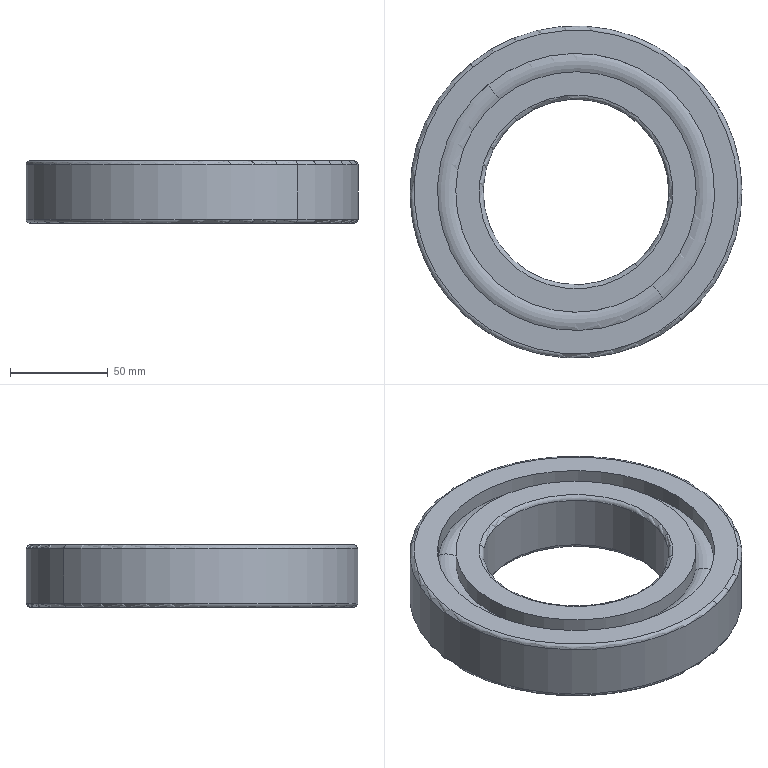Part | SolidWorks | features BaseBody 1 | 1 solid | 28 faces | box 170 x 170 x 32 mm | volume 443055 mm3 | cylinder 12 | torus 12 | plane 4 | commonest cylinder face diameters 123.125 x4 141.875 x4 95 x2 170 x2
STEP:
#1=CARTESIAN_POINT('',(467.199,300.361,-182.593));
#2=VERTEX_POINT('',#1);
#3=CARTESIAN_POINT('',(575.262,169.127,-182.593));
#4=VERTEX_POINT('',#3);
#5=CARTESIAN_POINT('',(521.231,234.744,-182.593));
#6=DIRECTION('',(0.,0.,1.));
#7=DIRECTION('',(-0.6357,0.772,0.));
#8=AXIS2_PLACEMENT_3D('',#5,#6,#7);
#9=CIRCLE('',#8,85.);
#10=EDGE_CURVE('',#2,#4,#9,.T.);
#11=ORIENTED_EDGE('',*,*,#10,.T.);
#12=CARTESIAN_POINT('',(575.262,169.127,-154.793));
#13=VERTEX_POINT('',#12);
#14=CARTESIAN_POINT('',(575.262,169.127,809.603));
#15=DIRECTION('',(0.,0.,1.));
#16=VECTOR('',#15,1000.);
#17=LINE('',#14,#16);
#18=EDGE_CURVE('',#4,#13,#17,.T.);
#19=ORIENTED_EDGE('',*,*,#18,.T.);
#20=CARTESIAN_POINT('',(467.199,300.361,-154.793));
#21=VERTEX_POINT('',#20);
#22=CARTESIAN_POINT('',(521.231,234.744,-154.793));
#23=DIRECTION('',(0.,0.,1.));
#24=DIRECTION('',(-0.6357,0.772,0.));
#25=AXIS2_PLACEMENT_3D('',#22,#23,#24);
#26=CIRCLE('',#25,85.);
#27=EDGE_CURVE('',#21,#13,#26,.T.);
#28=ORIENTED_EDGE('',*,*,#27,.F.);
#29=CARTESIAN_POINT('',(467.199,300.361,809.603));
#30=DIRECTION('',(0.,0.,1.));
#31=VECTOR('',#30,1000.);
#32=LINE('',#29,#31);
#33=EDGE_CURVE('',#2,#21,#32,.T.);
#34=ORIENTED_EDGE('',*,*,#33,.F.);
#35=EDGE_LOOP('',(#11,#19,#28,#34));
#36=FACE_OUTER_BOUND('',#35,.T.);
#37=CARTESIAN_POINT('',(521.231,234.744,809.603));
#38=DIRECTION('',(0.,0.,1.));
#39=DIRECTION('',(-0.6357,0.772,0.));
#40=AXIS2_PLACEMENT_3D('',#37,#38,#39);
#41=CYLINDRICAL_SURFACE('',#40,85.);
#42=ADVANCED_FACE('',(#36),#41,.T.);
#43=CARTESIAN_POINT('',(468.534,298.74,-184.693));
#44=VERTEX_POINT('',#43);
#45=CARTESIAN_POINT('',(573.928,170.748,-184.693));
#46=VERTEX_POINT('',#45);
#47=CARTESIAN_POINT('',(521.231,234.744,-184.693));
#48=DIRECTION('',(0.,0.,1.));
#49=DIRECTION('',(-0.6357,0.772,0.));
#50=AXIS2_PLACEMENT_3D('',#47,#48,#49);
#51=CIRCLE('',#50,82.9);
#52=EDGE_CURVE('',#44,#46,#51,.T.);
#53=ORIENTED_EDGE('',*,*,#52,.T.);
#54=CARTESIAN_POINT('',(573.928,170.748,-182.593));
#55=DIRECTION('',(-0.772,-0.6357,0.));
#56=DIRECTION('',(0.6357,-0.772,0.));
#57=AXIS2_PLACEMENT_3D('',#54,#55,#56);
#58=CIRCLE('',#57,2.1);
#59=EDGE_CURVE('',#46,#4,#58,.T.);
#60=ORIENTED_EDGE('',*,*,#59,.T.);
#61=ORIENTED_EDGE('',*,*,#10,.F.);
#62=CARTESIAN_POINT('',(468.534,298.74,-182.593));
#63=DIRECTION('',(0.772,0.6357,0.));
#64=DIRECTION('',(-0.6357,0.772,0.));
#65=AXIS2_PLACEMENT_3D('',#62,#63,#64);
#66=CIRCLE('',#65,2.1);
#67=EDGE_CURVE('',#44,#2,#66,.T.);
#68=ORIENTED_EDGE('',*,*,#67,.F.);
#69=EDGE_LOOP('',(#53,#60,#61,#68));
#70=FACE_OUTER_BOUND('',#69,.T.);
#71=CARTESIAN_POINT('',(521.231,234.744,-182.593));
#72=DIRECTION('',(0.,0.,1.));
#73=DIRECTION('',(-0.6357,0.772,0.));
#74=AXIS2_PLACEMENT_3D('',#71,#72,#73);
#75=TOROIDAL_SURFACE('',#74,82.9,2.1);
#76=ADVANCED_FACE('',(#70),#75,.T.);
#77=CARTESIAN_POINT('',(566.323,179.983,-184.693));
#78=VERTEX_POINT('',#77);
#79=CARTESIAN_POINT('',(476.138,289.505,-184.693));
#80=VERTEX_POINT('',#79);
#81=CARTESIAN_POINT('',(521.231,234.744,-184.693));
#82=DIRECTION('',(0.,0.,1.));
#83=DIRECTION('',(-0.6357,0.772,0.));
#84=AXIS2_PLACEMENT_3D('',#81,#82,#83);
#85=CIRCLE('',#84,70.938);
#86=EDGE_CURVE('',#78,#80,#85,.T.);
#87=ORIENTED_EDGE('',*,*,#86,.F.);
#88=CARTESIAN_POINT('',(566.323,179.983,-176.812));
#89=VERTEX_POINT('',#88);
#90=CARTESIAN_POINT('',(566.323,179.983,809.603));
#91=DIRECTION('',(0.,0.,1.));
#92=VECTOR('',#91,1000.);
#93=LINE('',#90,#92);
#94=EDGE_CURVE('',#78,#89,#93,.T.);
#95=ORIENTED_EDGE('',*,*,#94,.T.);
#96=CARTESIAN_POINT('',(476.138,289.505,-176.812));
#97=VERTEX_POINT('',#96);
#98=CARTESIAN_POINT('',(521.231,234.744,-176.812));
#99=DIRECTION('',(0.,0.,1.));
#100=DIRECTION('',(-0.6357,0.772,0.));
#101=AXIS2_PLACEMENT_3D('',#98,#99,#100);
#102=CIRCLE('',#101,70.938);
#103=EDGE_CURVE('',#89,#97,#102,.T.);
#104=ORIENTED_EDGE('',*,*,#103,.T.);
#105=CARTESIAN_POINT('',(476.138,289.505,809.603));
#106=DIRECTION('',(0.,0.,1.));
#107=VECTOR('',#106,1000.);
#108=LINE('',#105,#107);
#109=EDGE_CURVE('',#80,#97,#108,.T.);
#110=ORIENTED_EDGE('',*,*,#109,.F.);
#111=EDGE_LOOP('',(#87,#95,#104,#110));
#112=FACE_OUTER_BOUND('',#111,.T.);
#113=CARTESIAN_POINT('',(521.231,234.744,809.603));
#114=DIRECTION('',(0.,0.,1.));
#115=DIRECTION('',(-0.6357,0.772,0.));
#116=AXIS2_PLACEMENT_3D('',#113,#114,#115);
#117=CYLINDRICAL_SURFACE('',#116,70.938);
#118=ADVANCED_FACE('',(#112),#117,.F.);
#119=CARTESIAN_POINT('',(482.097,282.268,-176.812));
#120=VERTEX_POINT('',#119);
#121=CARTESIAN_POINT('',(560.364,187.22,-176.812));
#122=VERTEX_POINT('',#121);
#123=CARTESIAN_POINT('',(521.231,234.744,-176.812));
#124=DIRECTION('',(0.,0.,1.));
#125=DIRECTION('',(-0.6357,0.772,0.));
#126=AXIS2_PLACEMENT_3D('',#123,#124,#125);
#127=CIRCLE('',#126,61.563);
#128=EDGE_CURVE('',#120,#122,#127,.T.);
#129=ORIENTED_EDGE('',*,*,#128,.T.);
#130=CARTESIAN_POINT('',(563.344,183.601,-168.693));
#131=DIRECTION('',(-0.772,-0.6357,0.));
#132=DIRECTION('',(0.6357,-0.772,0.));
#133=AXIS2_PLACEMENT_3D('',#130,#131,#132);
#134=CIRCLE('',#133,9.375);
#135=EDGE_CURVE('',#122,#89,#134,.T.);
#136=ORIENTED_EDGE('',*,*,#135,.T.);
#137=CARTESIAN_POINT('',(521.231,234.744,-176.812));
#138=DIRECTION('',(0.,0.,1.));
#139=DIRECTION('',(-0.6357,0.772,0.));
#140=AXIS2_PLACEMENT_3D('',#137,#138,#139);
#141=CIRCLE('',#140,70.938);
#142=EDGE_CURVE('',#97,#89,#141,.T.);
#143=ORIENTED_EDGE('',*,*,#142,.F.);
#144=CARTESIAN_POINT('',(479.118,285.886,-168.693));
#145=DIRECTION('',(0.772,0.6357,0.));
#146=DIRECTION('',(-0.6357,0.772,0.));
#147=AXIS2_PLACEMENT_3D('',#144,#145,#146);
#148=CIRCLE('',#147,9.375);
#149=EDGE_CURVE('',#120,#97,#148,.T.);
#150=ORIENTED_EDGE('',*,*,#149,.F.);
#151=EDGE_LOOP('',(#129,#136,#143,#150));
#152=FACE_OUTER_BOUND('',#151,.T.);
#153=CARTESIAN_POINT('',(521.231,234.744,-168.693));
#154=DIRECTION('',(0.,0.,1.));
#155=DIRECTION('',(-0.6357,0.772,0.));
#156=AXIS2_PLACEMENT_3D('',#153,#154,#155);
#157=TOROIDAL_SURFACE('',#156,66.25,9.375);
#158=ADVANCED_FACE('',(#152),#157,.T.);
#159=CARTESIAN_POINT('',(482.097,282.268,-184.693));
#160=VERTEX_POINT('',#159);
#161=CARTESIAN_POINT('',(560.364,187.22,-184.693));
#162=VERTEX_POINT('',#161);
#163=CARTESIAN_POINT('',(521.231,234.744,-184.693));
#164=DIRECTION('',(0.,0.,1.));
#165=DIRECTION('',(-0.6357,0.772,0.));
#166=AXIS2_PLACEMENT_3D('',#163,#164,#165);
#167=CIRCLE('',#166,61.563);
#168=EDGE_CURVE('',#160,#162,#167,.T.);
#169=ORIENTED_EDGE('',*,*,#168,.T.);
#170=CARTESIAN_POINT('',(560.364,187.22,809.603));
#171=DIRECTION('',(0.,0.,1.));
#172=VECTOR('',#171,1000.);
#173=LINE('',#170,#172);
#174=EDGE_CURVE('',#162,#122,#173,.T.);
#175=ORIENTED_EDGE('',*,*,#174,.T.);
#176=ORIENTED_EDGE('',*,*,#128,.F.);
#177=CARTESIAN_POINT('',(482.097,282.268,809.603));
#178=DIRECTION('',(0.,0.,1.));
#179=VECTOR('',#178,1000.);
#180=LINE('',#177,#179);
#181=EDGE_CURVE('',#160,#120,#180,.T.);
#182=ORIENTED_EDGE('',*,*,#181,.F.);
#183=EDGE_LOOP('',(#169,#175,#176,#182));
#184=FACE_OUTER_BOUND('',#183,.T.);
#185=CARTESIAN_POINT('',(521.231,234.744,809.603));
#186=DIRECTION('',(0.,0.,1.));
#187=DIRECTION('',(-0.6357,0.772,0.));
#188=AXIS2_PLACEMENT_3D('',#185,#186,#187);
#189=CYLINDRICAL_SURFACE('',#188,61.563);
#190=ADVANCED_FACE('',(#184),#189,.T.);
#191=CARTESIAN_POINT('',(491.036,271.412,-182.593));
#192=VERTEX_POINT('',#191);
#193=CARTESIAN_POINT('',(551.425,198.076,-182.593));
#194=VERTEX_POINT('',#193);
#195=CARTESIAN_POINT('',(521.231,234.744,-182.593));
#196=DIRECTION('',(0.,0.,1.));
#197=DIRECTION('',(-0.6357,0.772,0.));
#198=AXIS2_PLACEMENT_3D('',#195,#196,#197);
#199=CIRCLE('',#198,47.5);
#200=EDGE_CURVE('',#192,#194,#199,.T.);
#201=ORIENTED_EDGE('',*,*,#200,.T.);
#202=CARTESIAN_POINT('',(552.76,196.455,-184.693));
#203=VERTEX_POINT('',#202);
#204=CARTESIAN_POINT('',(552.76,196.455,-182.593));
#205=DIRECTION('',(-0.772,-0.6357,0.));
#206=DIRECTION('',(0.6357,-0.772,0.));
#207=AXIS2_PLACEMENT_3D('',#204,#205,#206);
#208=CIRCLE('',#207,2.1);
#209=EDGE_CURVE('',#194,#203,#208,.T.);
#210=ORIENTED_EDGE('',*,*,#209,.T.);
#211=CARTESIAN_POINT('',(489.701,273.033,-184.693));
#212=VERTEX_POINT('',#211);
#213=CARTESIAN_POINT('',(521.231,234.744,-184.693));
#214=DIRECTION('',(0.,0.,1.));
#215=DIRECTION('',(-0.6357,0.772,0.));
#216=AXIS2_PLACEMENT_3D('',#213,#214,#215);
#217=CIRCLE('',#216,49.6);
#218=EDGE_CURVE('',#212,#203,#217,.T.);
#219=ORIENTED_EDGE('',*,*,#218,.F.);
#220=CARTESIAN_POINT('',(489.701,273.033,-182.593));
#221=DIRECTION('',(0.772,0.6357,0.));
#222=DIRECTION('',(-0.6357,0.772,0.));
#223=AXIS2_PLACEMENT_3D('',#220,#221,#222);
#224=CIRCLE('',#223,2.1);
#225=EDGE_CURVE('',#192,#212,#224,.T.);
#226=ORIENTED_EDGE('',*,*,#225,.F.);
#227=EDGE_LOOP('',(#201,#210,#219,#226));
#228=FACE_OUTER_BOUND('',#227,.T.);
#229=CARTESIAN_POINT('',(521.231,234.744,-182.593));
#230=DIRECTION('',(0.,0.,1.));
#231=DIRECTION('',(-0.6357,0.772,0.));
#232=AXIS2_PLACEMENT_3D('',#229,#230,#231);
#233=TOROIDAL_SURFACE('',#232,49.6,2.1);
#234=ADVANCED_FACE('',(#228),#233,.T.);
#235=CARTESIAN_POINT('',(521.231,234.744,-182.593));
#236=DIRECTION('',(0.,0.,1.));
#237=DIRECTION('',(-0.6357,0.772,0.));
#238=AXIS2_PLACEMENT_3D('',#235,#236,#237);
#239=CIRCLE('',#238,47.5);
#240=EDGE_CURVE('',#194,#192,#239,.T.);
#241=ORIENTED_EDGE('',*,*,#240,.F.);
#242=CARTESIAN_POINT('',(551.425,198.076,-154.793));
#243=VERTEX_POINT('',#242);
#244=CARTESIAN_POINT('',(551.425,198.076,809.603));
#245=DIRECTION('',(0.,0.,1.));
#246=VECTOR('',#245,1000.);
#247=LINE('',#244,#246);
#248=EDGE_CURVE('',#194,#243,#247,.T.);
#249=ORIENTED_EDGE('',*,*,#248,.T.);
#250=CARTESIAN_POINT('',(491.036,271.412,-154.793));
#251=VERTEX_POINT('',#250);
#252=CARTESIAN_POINT('',(521.231,234.744,-154.793));
#253=DIRECTION('',(0.,0.,1.));
#254=DIRECTION('',(-0.6357,0.772,0.));
#255=AXIS2_PLACEMENT_3D('',#252,#253,#254);
#256=CIRCLE('',#255,47.5);
#257=EDGE_CURVE('',#243,#251,#256,.T.);
#258=ORIENTED_EDGE('',*,*,#257,.T.);
#259=CARTESIAN_POINT('',(491.036,271.412,809.603));
#260=DIRECTION('',(0.,0.,1.));
#261=VECTOR('',#260,1000.);
#262=LINE('',#259,#261);
#263=EDGE_CURVE('',#192,#251,#262,.T.);
#264=ORIENTED_EDGE('',*,*,#263,.F.);
#265=EDGE_LOOP('',(#241,#249,#258,#264));
#266=FACE_OUTER_BOUND('',#265,.T.);
#267=CARTESIAN_POINT('',(521.231,234.744,809.603));
#268=DIRECTION('',(0.,0.,1.));
#269=DIRECTION('',(-0.6357,0.772,0.));
#270=AXIS2_PLACEMENT_3D('',#267,#268,#269);
#271=CYLINDRICAL_SURFACE('',#270,47.5);
#272=ADVANCED_FACE('',(#266),#271,.F.);
#273=CARTESIAN_POINT('',(489.701,273.033,-152.693));
#274=VERTEX_POINT('',#273);
#275=CARTESIAN_POINT('',(552.76,196.455,-152.693));
#276=VERTEX_POINT('',#275);
#277=CARTESIAN_POINT('',(521.231,234.744,-152.693));
#278=DIRECTION('',(0.,0.,1.));
#279=DIRECTION('',(-0.6357,0.772,0.));
#280=AXIS2_PLACEMENT_3D('',#277,#278,#279);
#281=CIRCLE('',#280,49.6);
#282=EDGE_CURVE('',#274,#276,#281,.T.);
#283=ORIENTED_EDGE('',*,*,#282,.T.);
#284=CARTESIAN_POINT('',(552.76,196.455,-154.793));
#285=DIRECTION('',(-0.772,-0.6357,0.));
#286=DIRECTION('',(0.6357,-0.772,0.));
#287=AXIS2_PLACEMENT_3D('',#284,#285,#286);
#288=CIRCLE('',#287,2.1);
#289=EDGE_CURVE('',#276,#243,#288,.T.);
#290=ORIENTED_EDGE('',*,*,#289,.T.);
#291=CARTESIAN_POINT('',(521.231,234.744,-154.793));
#292=DIRECTION('',(0.,0.,1.));
#293=DIRECTION('',(-0.6357,0.772,0.));
#294=AXIS2_PLACEMENT_3D('',#291,#292,#293);
#295=CIRCLE('',#294,47.5);
#296=EDGE_CURVE('',#251,#243,#295,.T.);
#297=ORIENTED_EDGE('',*,*,#296,.F.);
#298=CARTESIAN_POINT('',(489.701,273.033,-154.793));
#299=DIRECTION('',(0.772,0.6357,0.));
#300=DIRECTION('',(-0.6357,0.772,0.));
#301=AXIS2_PLACEMENT_3D('',#298,#299,#300);
#302=CIRCLE('',#301,2.1);
#303=EDGE_CURVE('',#274,#251,#302,.T.);
#304=ORIENTED_EDGE('',*,*,#303,.F.);
#305=EDGE_LOOP('',(#283,#290,#297,#304));
#306=FACE_OUTER_BOUND('',#305,.T.);
#307=CARTESIAN_POINT('',(521.231,234.744,-154.793));
#308=DIRECTION('',(0.,0.,1.));
#309=DIRECTION('',(-0.6357,0.772,0.));
#310=AXIS2_PLACEMENT_3D('',#307,#308,#309);
#311=TOROIDAL_SURFACE('',#310,49.6,2.1);
#312=ADVANCED_FACE('',(#306),#311,.T.);
#313=CARTESIAN_POINT('',(482.097,282.268,-160.574));
#314=VERTEX_POINT('',#313);
#315=CARTESIAN_POINT('',(560.364,187.22,-160.574));
#316=VERTEX_POINT('',#315);
#317=CARTESIAN_POINT('',(521.231,234.744,-160.574));
#318=DIRECTION('',(0.,0.,1.));
#319=DIRECTION('',(-0.6357,0.772,0.));
#320=AXIS2_PLACEMENT_3D('',#317,#318,#319);
#321=CIRCLE('',#320,61.563);
#322=EDGE_CURVE('',#314,#316,#321,.T.);
#323=ORIENTED_EDGE('',*,*,#322,.T.);
#324=CARTESIAN_POINT('',(560.364,187.22,-152.693));
#325=VERTEX_POINT('',#324);
#326=CARTESIAN_POINT('',(560.364,187.22,809.603));
#327=DIRECTION('',(0.,0.,1.));
#328=VECTOR('',#327,1000.);
#329=LINE('',#326,#328);
#330=EDGE_CURVE('',#316,#325,#329,.T.);
#331=ORIENTED_EDGE('',*,*,#330,.T.);
#332=CARTESIAN_POINT('',(482.097,282.268,-152.693));
#333=VERTEX_POINT('',#332);
#334=CARTESIAN_POINT('',(521.231,234.744,-152.693));
#335=DIRECTION('',(0.,0.,1.));
#336=DIRECTION('',(-0.6357,0.772,0.));
#337=AXIS2_PLACEMENT_3D('',#334,#335,#336);
#338=CIRCLE('',#337,61.563);
#339=EDGE_CURVE('',#333,#325,#338,.T.);
#340=ORIENTED_EDGE('',*,*,#339,.F.);
#341=CARTESIAN_POINT('',(482.097,282.268,809.603));
#342=DIRECTION('',(0.,0.,1.));
#343=VECTOR('',#342,1000.);
#344=LINE('',#341,#343);
#345=EDGE_CURVE('',#314,#333,#344,.T.);
#346=ORIENTED_EDGE('',*,*,#345,.F.);
#347=EDGE_LOOP('',(#323,#331,#340,#346));
#348=FACE_OUTER_BOUND('',#347,.T.);
#349=CARTESIAN_POINT('',(521.231,234.744,809.603));
#350=DIRECTION('',(0.,0.,1.));
#351=DIRECTION('',(-0.6357,0.772,0.));
#352=AXIS2_PLACEMENT_3D('',#349,#350,#351);
#353=CYLINDRICAL_SURFACE('',#352,61.563);
#354=ADVANCED_FACE('',(#348),#353,.T.);
#355=CARTESIAN_POINT('',(476.138,289.505,-160.574));
#356=VERTEX_POINT('',#355);
#357=CARTESIAN_POINT('',(566.323,179.983,-160.574));
#358=VERTEX_POINT('',#357);
#359=CARTESIAN_POINT('',(521.231,234.744,-160.574));
#360=DIRECTION('',(0.,0.,1.));
#361=DIRECTION('',(-0.6357,0.772,0.));
#362=AXIS2_PLACEMENT_3D('',#359,#360,#361);
#363=CIRCLE('',#362,70.938);
#364=EDGE_CURVE('',#356,#358,#363,.T.);
#365=ORIENTED_EDGE('',*,*,#364,.T.);
#366=CARTESIAN_POINT('',(563.344,183.601,-168.693));
#367=DIRECTION('',(-0.772,-0.6357,0.));
#368=DIRECTION('',(0.6357,-0.772,0.));
#369=AXIS2_PLACEMENT_3D('',#366,#367,#368);
#370=CIRCLE('',#369,9.375);
#371=EDGE_CURVE('',#358,#316,#370,.T.);
#372=ORIENTED_EDGE('',*,*,#371,.T.);
#373=ORIENTED_EDGE('',*,*,#322,.F.);
#374=CARTESIAN_POINT('',(479.118,285.886,-168.693));
#375=DIRECTION('',(0.772,0.6357,0.));
#376=DIRECTION('',(-0.6357,0.772,0.));
#377=AXIS2_PLACEMENT_3D('',#374,#375,#376);
#378=CIRCLE('',#377,9.375);
#379=EDGE_CURVE('',#356,#314,#378,.T.);
#380=ORIENTED_EDGE('',*,*,#379,.F.);
#381=EDGE_LOOP('',(#365,#372,#373,#380));
#382=FACE_OUTER_BOUND('',#381,.T.);
#383=CARTESIAN_POINT('',(521.231,234.744,-168.693));
#384=DIRECTION('',(0.,0.,1.));
#385=DIRECTION('',(-0.6357,0.772,0.));
#386=AXIS2_PLACEMENT_3D('',#383,#384,#385);
#387=TOROIDAL_SURFACE('',#386,66.25,9.375);
#388=ADVANCED_FACE('',(#382),#387,.T.);
#389=CARTESIAN_POINT('',(521.231,234.744,-160.574));
#390=DIRECTION('',(0.,0.,1.));
#391=DIRECTION('',(-0.6357,0.772,0.));
#392=AXIS2_PLACEMENT_3D('',#389,#390,#391);
#393=CIRCLE('',#392,70.938);
#394=EDGE_CURVE('',#358,#356,#393,.T.);
#395=ORIENTED_EDGE('',*,*,#394,.F.);
#396=CARTESIAN_POINT('',(566.323,179.983,-152.693));
#397=VERTEX_POINT('',#396);
#398=CARTESIAN_POINT('',(566.323,179.983,809.603));
#399=DIRECTION('',(0.,0.,1.));
#400=VECTOR('',#399,1000.);
#401=LINE('',#398,#400);
#402=EDGE_CURVE('',#358,#397,#401,.T.);
#403=ORIENTED_EDGE('',*,*,#402,.T.);
#404=CARTESIAN_POINT('',(476.138,289.505,-152.693));
#405=VERTEX_POINT('',#404);
#406=CARTESIAN_POINT('',(521.231,234.744,-152.693));
#407=DIRECTION('',(0.,0.,1.));
#408=DIRECTION('',(-0.6357,0.772,0.));
#409=AXIS2_PLACEMENT_3D('',#406,#407,#408);
#410=CIRCLE('',#409,70.938);
#411=EDGE_CURVE('',#397,#405,#410,.T.);
#412=ORIENTED_EDGE('',*,*,#411,.T.);
#413=CARTESIAN_POINT('',(476.138,289.505,809.603));
#414=DIRECTION('',(0.,0.,1.));
#415=VECTOR('',#414,1000.);
#416=LINE('',#413,#415);
#417=EDGE_CURVE('',#356,#405,#416,.T.);
#418=ORIENTED_EDGE('',*,*,#417,.F.);
#419=EDGE_LOOP('',(#395,#403,#412,#418));
#420=FACE_OUTER_BOUND('',#419,.T.);
#421=CARTESIAN_POINT('',(521.231,234.744,809.603));
#422=DIRECTION('',(0.,0.,1.));
#423=DIRECTION('',(-0.6357,0.772,0.));
#424=AXIS2_PLACEMENT_3D('',#421,#422,#423);
#425=CYLINDRICAL_SURFACE('',#424,70.938);
#426=ADVANCED_FACE('',(#420),#425,.F.);
#427=ORIENTED_EDGE('',*,*,#27,.T.);
#428=CARTESIAN_POINT('',(573.928,170.748,-152.693));
#429=VERTEX_POINT('',#428);
#430=CARTESIAN_POINT('',(573.928,170.748,-154.793));
#431=DIRECTION('',(-0.772,-0.6357,0.));
#432=DIRECTION('',(0.6357,-0.772,0.));
#433=AXIS2_PLACEMENT_3D('',#430,#431,#432);
#434=CIRCLE('',#433,2.1);
#435=EDGE_CURVE('',#13,#429,#434,.T.);
#436=ORIENTED_EDGE('',*,*,#435,.T.);
#437=CARTESIAN_POINT('',(468.534,298.74,-152.693));
#438=VERTEX_POINT('',#437);
#439=CARTESIAN_POINT('',(521.231,234.744,-152.693));
#440=DIRECTION('',(0.,0.,1.));
#441=DIRECTION('',(-0.6357,0.772,0.));
#442=AXIS2_PLACEMENT_3D('',#439,#440,#441);
#443=CIRCLE('',#442,82.9);
#444=EDGE_CURVE('',#438,#429,#443,.T.);
#445=ORIENTED_EDGE('',*,*,#444,.F.);
#446=CARTESIAN_POINT('',(468.534,298.74,-154.793));
#447=DIRECTION('',(0.772,0.6357,0.));
#448=DIRECTION('',(-0.6357,0.772,0.));
#449=AXIS2_PLACEMENT_3D('',#446,#447,#448);
#450=CIRCLE('',#449,2.1);
#451=EDGE_CURVE('',#21,#438,#450,.T.);
#452=ORIENTED_EDGE('',*,*,#451,.F.);
#453=EDGE_LOOP('',(#427,#436,#445,#452));
#454=FACE_OUTER_BOUND('',#453,.T.);
#455=CARTESIAN_POINT('',(521.231,234.744,-154.793));
#456=DIRECTION('',(0.,0.,1.));
#457=DIRECTION('',(-0.6357,0.772,0.));
#458=AXIS2_PLACEMENT_3D('',#455,#456,#457);
#459=TOROIDAL_SURFACE('',#458,82.9,2.1);
#460=ADVANCED_FACE('',(#454),#459,.T.);
#461=ORIENTED_EDGE('',*,*,#435,.F.);
#462=CARTESIAN_POINT('',(521.231,234.744,-154.793));
#463=DIRECTION('',(0.,0.,1.));
#464=DIRECTION('',(-0.6357,0.772,0.));
#465=AXIS2_PLACEMENT_3D('',#462,#463,#464);
#466=CIRCLE('',#465,85.);
#467=EDGE_CURVE('',#13,#21,#466,.T.);
#468=ORIENTED_EDGE('',*,*,#467,.T.);
#469=ORIENTED_EDGE('',*,*,#451,.T.);
#470=CARTESIAN_POINT('',(521.231,234.744,-152.693));
#471=DIRECTION('',(0.,0.,1.));
#472=DIRECTION('',(-0.6357,0.772,0.));
#473=AXIS2_PLACEMENT_3D('',#470,#471,#472);
#474=CIRCLE('',#473,82.9);
#475=EDGE_CURVE('',#429,#438,#474,.T.);
#476=ORIENTED_EDGE('',*,*,#475,.F.);
#477=EDGE_LOOP('',(#461,#468,#469,#476));
#478=FACE_OUTER_BOUND('',#477,.T.);
#479=CARTESIAN_POINT('',(521.231,234.744,-154.793));
#480=DIRECTION('',(0.,0.,1.));
#481=DIRECTION('',(-0.6357,0.772,0.));
#482=AXIS2_PLACEMENT_3D('',#479,#480,#481);
#483=TOROIDAL_SURFACE('',#482,82.9,2.1);
#484=ADVANCED_FACE('',(#478),#483,.T.);
#485=CARTESIAN_POINT('',(521.231,234.744,-152.693));
#486=DIRECTION('',(0.,0.,1.));
#487=DIRECTION('',(-0.6357,0.772,0.));
#488=AXIS2_PLACEMENT_3D('',#485,#486,#487);
#489=CIRCLE('',#488,70.938);
#490=EDGE_CURVE('',#405,#397,#489,.T.);
#491=ORIENTED_EDGE('',*,*,#490,.F.);
#492=ORIENTED_EDGE('',*,*,#411,.F.);
#493=EDGE_LOOP('',(#491,#492));
#494=FACE_BOUND('',#493,.T.);
#495=ORIENTED_EDGE('',*,*,#444,.T.);
#496=ORIENTED_EDGE('',*,*,#475,.T.);
#497=EDGE_LOOP('',(#495,#496));
#498=FACE_OUTER_BOUND('',#497,.T.);
#499=CARTESIAN_POINT('',(457.235,182.047,-152.693));
#500=DIRECTION('',(0.,0.,-1.));
#501=DIRECTION('',(0.6357,-0.772,0.));
#502=AXIS2_PLACEMENT_3D('',#499,#500,#501);
#503=PLANE('',#502);
#504=ADVANCED_FACE('',(#494,#498),#503,.F.);
#505=ORIENTED_EDGE('',*,*,#402,.F.);
#506=ORIENTED_EDGE('',*,*,#364,.F.);
#507=ORIENTED_EDGE('',*,*,#417,.T.);
#508=ORIENTED_EDGE('',*,*,#490,.T.);
#509=EDGE_LOOP('',(#505,#506,#507,#508));
#510=FACE_OUTER_BOUND('',#509,.T.);
#511=CARTESIAN_POINT('',(521.231,234.744,809.603));
#512=DIRECTION('',(0.,0.,1.));
#513=DIRECTION('',(-0.6357,0.772,0.));
#514=AXIS2_PLACEMENT_3D('',#511,#512,#513);
#515=CYLINDRICAL_SURFACE('',#514,70.938);
#516=ADVANCED_FACE('',(#510),#515,.F.);
#517=ORIENTED_EDGE('',*,*,#371,.F.);
#518=ORIENTED_EDGE('',*,*,#394,.T.);
#519=ORIENTED_EDGE('',*,*,#379,.T.);
#520=CARTESIAN_POINT('',(521.231,234.744,-160.574));
#521=DIRECTION('',(0.,0.,1.));
#522=DIRECTION('',(-0.6357,0.772,0.));
#523=AXIS2_PLACEMENT_3D('',#520,#521,#522);
#524=CIRCLE('',#523,61.563);
#525=EDGE_CURVE('',#316,#314,#524,.T.);
#526=ORIENTED_EDGE('',*,*,#525,.F.);
#527=EDGE_LOOP('',(#517,#518,#519,#526));
#528=FACE_OUTER_BOUND('',#527,.T.);
#529=CARTESIAN_POINT('',(521.231,234.744,-168.693));
#530=DIRECTION('',(0.,0.,1.));
#531=DIRECTION('',(-0.6357,0.772,0.));
#532=AXIS2_PLACEMENT_3D('',#529,#530,#531);
#533=TOROIDAL_SURFACE('',#532,66.25,9.375);
#534=ADVANCED_FACE('',(#528),#533,.T.);
#535=ORIENTED_EDGE('',*,*,#330,.F.);
#536=ORIENTED_EDGE('',*,*,#525,.T.);
#537=ORIENTED_EDGE('',*,*,#345,.T.);
#538=CARTESIAN_POINT('',(521.231,234.744,-152.693));
#539=DIRECTION('',(0.,0.,1.));
#540=DIRECTION('',(-0.6357,0.772,0.));
#541=AXIS2_PLACEMENT_3D('',#538,#539,#540);
#542=CIRCLE('',#541,61.563);
#543=EDGE_CURVE('',#325,#333,#542,.T.);
#544=ORIENTED_EDGE('',*,*,#543,.F.);
#545=EDGE_LOOP('',(#535,#536,#537,#544));
#546=FACE_OUTER_BOUND('',#545,.T.);
#547=CARTESIAN_POINT('',(521.231,234.744,809.603));
#548=DIRECTION('',(0.,0.,1.));
#549=DIRECTION('',(-0.6357,0.772,0.));
#550=AXIS2_PLACEMENT_3D('',#547,#548,#549);
#551=CYLINDRICAL_SURFACE('',#550,61.563);
#552=ADVANCED_FACE('',(#546),#551,.T.);
#553=ORIENTED_EDGE('',*,*,#282,.F.);
#554=CARTESIAN_POINT('',(521.231,234.744,-152.693));
#555=DIRECTION('',(0.,0.,1.));
#556=DIRECTION('',(-0.6357,0.772,0.));
#557=AXIS2_PLACEMENT_3D('',#554,#555,#556);
#558=CIRCLE('',#557,49.6);
#559=EDGE_CURVE('',#276,#274,#558,.T.);
#560=ORIENTED_EDGE('',*,*,#559,.F.);
#561=EDGE_LOOP('',(#553,#560));
#562=FACE_BOUND('',#561,.T.);
#563=ORIENTED_EDGE('',*,*,#339,.T.);
#564=ORIENTED_EDGE('',*,*,#543,.T.);
#565=EDGE_LOOP('',(#563,#564));
#566=FACE_OUTER_BOUND('',#565,.T.);
#567=CARTESIAN_POINT('',(473.707,195.611,-152.693));
#568=DIRECTION('',(0.,0.,-1.));
#569=DIRECTION('',(0.6357,-0.772,0.));
#570=AXIS2_PLACEMENT_3D('',#567,#568,#569);
#571=PLANE('',#570);
#572=ADVANCED_FACE('',(#562,#566),#571,.F.);
#573=ORIENTED_EDGE('',*,*,#289,.F.);
#574=ORIENTED_EDGE('',*,*,#559,.T.);
#575=ORIENTED_EDGE('',*,*,#303,.T.);
#576=ORIENTED_EDGE('',*,*,#257,.F.);
#577=EDGE_LOOP('',(#573,#574,#575,#576));
#578=FACE_OUTER_BOUND('',#577,.T.);
#579=CARTESIAN_POINT('',(521.231,234.744,-154.793));
#580=DIRECTION('',(0.,0.,1.));
#581=DIRECTION('',(-0.6357,0.772,0.));
#582=AXIS2_PLACEMENT_3D('',#579,#580,#581);
#583=TOROIDAL_SURFACE('',#582,49.6,2.1);
#584=ADVANCED_FACE('',(#578),#583,.T.);
#585=ORIENTED_EDGE('',*,*,#248,.F.);
#586=ORIENTED_EDGE('',*,*,#200,.F.);
#587=ORIENTED_EDGE('',*,*,#263,.T.);
#588=ORIENTED_EDGE('',*,*,#296,.T.);
#589=EDGE_LOOP('',(#585,#586,#587,#588));
#590=FACE_OUTER_BOUND('',#589,.T.);
#591=CARTESIAN_POINT('',(521.231,234.744,809.603));
#592=DIRECTION('',(0.,0.,1.));
#593=DIRECTION('',(-0.6357,0.772,0.));
#594=AXIS2_PLACEMENT_3D('',#591,#592,#593);
#595=CYLINDRICAL_SURFACE('',#594,47.5);
#596=ADVANCED_FACE('',(#590),#595,.F.);
#597=ORIENTED_EDGE('',*,*,#209,.F.);
#598=ORIENTED_EDGE('',*,*,#240,.T.);
#599=ORIENTED_EDGE('',*,*,#225,.T.);
#600=CARTESIAN_POINT('',(521.231,234.744,-184.693));
#601=DIRECTION('',(0.,0.,1.));
#602=DIRECTION('',(-0.6357,0.772,0.));
#603=AXIS2_PLACEMENT_3D('',#600,#601,#602);
#604=CIRCLE('',#603,49.6);
#605=EDGE_CURVE('',#203,#212,#604,.T.);
#606=ORIENTED_EDGE('',*,*,#605,.F.);
#607=EDGE_LOOP('',(#597,#598,#599,#606));
#608=FACE_OUTER_BOUND('',#607,.T.);
#609=CARTESIAN_POINT('',(521.231,234.744,-182.593));
#610=DIRECTION('',(0.,0.,1.));
#611=DIRECTION('',(-0.6357,0.772,0.));
#612=AXIS2_PLACEMENT_3D('',#609,#610,#611);
#613=TOROIDAL_SURFACE('',#612,49.6,2.1);
#614=ADVANCED_FACE('',(#608),#613,.T.);
#615=ORIENTED_EDGE('',*,*,#168,.F.);
#616=CARTESIAN_POINT('',(521.231,234.744,-184.693));
#617=DIRECTION('',(0.,0.,1.));
#618=DIRECTION('',(-0.6357,0.772,0.));
#619=AXIS2_PLACEMENT_3D('',#616,#617,#618);
#620=CIRCLE('',#619,61.563);
#621=EDGE_CURVE('',#162,#160,#620,.T.);
#622=ORIENTED_EDGE('',*,*,#621,.F.);
#623=EDGE_LOOP('',(#615,#622));
#624=FACE_OUTER_BOUND('',#623,.T.);
#625=ORIENTED_EDGE('',*,*,#218,.T.);
#626=ORIENTED_EDGE('',*,*,#605,.T.);
#627=EDGE_LOOP('',(#625,#626));
#628=FACE_BOUND('',#627,.T.);
#629=CARTESIAN_POINT('',(473.707,195.611,-184.693));
#630=DIRECTION('',(0.,0.,1.));
#631=DIRECTION('',(-0.6357,0.772,0.));
#632=AXIS2_PLACEMENT_3D('',#629,#630,#631);
#633=PLANE('',#632);
#634=ADVANCED_FACE('',(#624,#628),#633,.F.);
#635=ORIENTED_EDGE('',*,*,#174,.F.);
#636=ORIENTED_EDGE('',*,*,#621,.T.);
#637=ORIENTED_EDGE('',*,*,#181,.T.);
#638=CARTESIAN_POINT('',(521.231,234.744,-176.812));
#639=DIRECTION('',(0.,0.,1.));
#640=DIRECTION('',(-0.6357,0.772,0.));
#641=AXIS2_PLACEMENT_3D('',#638,#639,#640);
#642=CIRCLE('',#641,61.563);
#643=EDGE_CURVE('',#122,#120,#642,.T.);
#644=ORIENTED_EDGE('',*,*,#643,.F.);
#645=EDGE_LOOP('',(#635,#636,#637,#644));
#646=FACE_OUTER_BOUND('',#645,.T.);
#647=CARTESIAN_POINT('',(521.231,234.744,809.603));
#648=DIRECTION('',(0.,0.,1.));
#649=DIRECTION('',(-0.6357,0.772,0.));
#650=AXIS2_PLACEMENT_3D('',#647,#648,#649);
#651=CYLINDRICAL_SURFACE('',#650,61.563);
#652=ADVANCED_FACE('',(#646),#651,.T.);
#653=ORIENTED_EDGE('',*,*,#135,.F.);
#654=ORIENTED_EDGE('',*,*,#643,.T.);
#655=ORIENTED_EDGE('',*,*,#149,.T.);
#656=ORIENTED_EDGE('',*,*,#103,.F.);
#657=EDGE_LOOP('',(#653,#654,#655,#656));
#658=FACE_OUTER_BOUND('',#657,.T.);
#659=CARTESIAN_POINT('',(521.231,234.744,-168.693));
#660=DIRECTION('',(0.,0.,1.));
#661=DIRECTION('',(-0.6357,0.772,0.));
#662=AXIS2_PLACEMENT_3D('',#659,#660,#661);
#663=TOROIDAL_SURFACE('',#662,66.25,9.375);
#664=ADVANCED_FACE('',(#658),#663,.T.);
#665=ORIENTED_EDGE('',*,*,#94,.F.);
#666=CARTESIAN_POINT('',(521.231,234.744,-184.693));
#667=DIRECTION('',(0.,0.,1.));
#668=DIRECTION('',(-0.6357,0.772,0.));
#669=AXIS2_PLACEMENT_3D('',#666,#667,#668);
#670=CIRCLE('',#669,70.938);
#671=EDGE_CURVE('',#80,#78,#670,.T.);
#672=ORIENTED_EDGE('',*,*,#671,.F.);
#673=ORIENTED_EDGE('',*,*,#109,.T.);
#674=ORIENTED_EDGE('',*,*,#142,.T.);
#675=EDGE_LOOP('',(#665,#672,#673,#674));
#676=FACE_OUTER_BOUND('',#675,.T.);
#677=CARTESIAN_POINT('',(521.231,234.744,809.603));
#678=DIRECTION('',(0.,0.,1.));
#679=DIRECTION('',(-0.6357,0.772,0.));
#680=AXIS2_PLACEMENT_3D('',#677,#678,#679);
#681=CYLINDRICAL_SURFACE('',#680,70.938);
#682=ADVANCED_FACE('',(#676),#681,.F.);
#683=ORIENTED_EDGE('',*,*,#52,.F.);
#684=CARTESIAN_POINT('',(521.231,234.744,-184.693));
#685=DIRECTION('',(0.,0.,1.));
#686=DIRECTION('',(-0.6357,0.772,0.));
#687=AXIS2_PLACEMENT_3D('',#684,#685,#686);
#688=CIRCLE('',#687,82.9);
#689=EDGE_CURVE('',#46,#44,#688,.T.);
#690=ORIENTED_EDGE('',*,*,#689,.F.);
#691=EDGE_LOOP('',(#683,#690));
#692=FACE_OUTER_BOUND('',#691,.T.);
#693=ORIENTED_EDGE('',*,*,#671,.T.);
#694=ORIENTED_EDGE('',*,*,#86,.T.);
#695=EDGE_LOOP('',(#693,#694));
#696=FACE_BOUND('',#695,.T.);
#697=CARTESIAN_POINT('',(457.235,182.047,-184.693));
#698=DIRECTION('',(0.,0.,1.));
#699=DIRECTION('',(-0.6357,0.772,0.));
#700=AXIS2_PLACEMENT_3D('',#697,#698,#699);
#701=PLANE('',#700);
#702=ADVANCED_FACE('',(#692,#696),#701,.F.);
#703=ORIENTED_EDGE('',*,*,#59,.F.);
#704=ORIENTED_EDGE('',*,*,#689,.T.);
#705=ORIENTED_EDGE('',*,*,#67,.T.);
#706=CARTESIAN_POINT('',(521.231,234.744,-182.593));
#707=DIRECTION('',(0.,0.,1.));
#708=DIRECTION('',(-0.6357,0.772,0.));
#709=AXIS2_PLACEMENT_3D('',#706,#707,#708);
#710=CIRCLE('',#709,85.);
#711=EDGE_CURVE('',#4,#2,#710,.T.);
#712=ORIENTED_EDGE('',*,*,#711,.F.);
#713=EDGE_LOOP('',(#703,#704,#705,#712));
#714=FACE_OUTER_BOUND('',#713,.T.);
#715=CARTESIAN_POINT('',(521.231,234.744,-182.593));
#716=DIRECTION('',(0.,0.,1.));
#717=DIRECTION('',(-0.6357,0.772,0.));
#718=AXIS2_PLACEMENT_3D('',#715,#716,#717);
#719=TOROIDAL_SURFACE('',#718,82.9,2.1);
#720=ADVANCED_FACE('',(#714),#719,.T.);
#721=ORIENTED_EDGE('',*,*,#18,.F.);
#722=ORIENTED_EDGE('',*,*,#711,.T.);
#723=ORIENTED_EDGE('',*,*,#33,.T.);
#724=ORIENTED_EDGE('',*,*,#467,.F.);
#725=EDGE_LOOP('',(#721,#722,#723,#724));
#726=FACE_OUTER_BOUND('',#725,.T.);
#727=CARTESIAN_POINT('',(521.231,234.744,809.603));
#728=DIRECTION('',(0.,0.,1.));
#729=DIRECTION('',(-0.6357,0.772,0.));
#730=AXIS2_PLACEMENT_3D('',#727,#728,#729);
#731=CYLINDRICAL_SURFACE('',#730,85.);
#732=ADVANCED_FACE('',(#726),#731,.T.);
#733=CLOSED_SHELL('',(#42,#76,#118,#158,#190,#234,#272,#312,#354,#388,#426,#460,#484,#504,#516,#534,#552,#572,#584,#596,#614,#634,#652,#664,#682,#702,#720,#732));
#734=MANIFOLD_SOLID_BREP('',#733);
#735=CARTESIAN_POINT('',(0.,0.,0.));
#736=DIRECTION('',(0.,0.,1.));
#737=DIRECTION('',(1.,0.,0.));
#738=AXIS2_PLACEMENT_3D('',#735,#736,#737);
#739=(LENGTH_UNIT()NAMED_UNIT(*)SI_UNIT(.MILLI.,.METRE.));
#740=UNCERTAINTY_MEASURE_WITH_UNIT(LENGTH_MEASURE(0.00001),#739,'','');
#741=(NAMED_UNIT(*)PLANE_ANGLE_UNIT()SI_UNIT($,.RADIAN.));
#742=(NAMED_UNIT(*)SI_UNIT($,.STERADIAN.)SOLID_ANGLE_UNIT());
#743=(GEOMETRIC_REPRESENTATION_CONTEXT(3)GLOBAL_UNCERTAINTY_ASSIGNED_CONTEXT((#740))GLOBAL_UNIT_ASSIGNED_CONTEXT((#739,#741,#742))REPRESENTATION_CONTEXT('',''));
#744=ADVANCED_BREP_SHAPE_REPRESENTATION('',(#734,#738),#743);